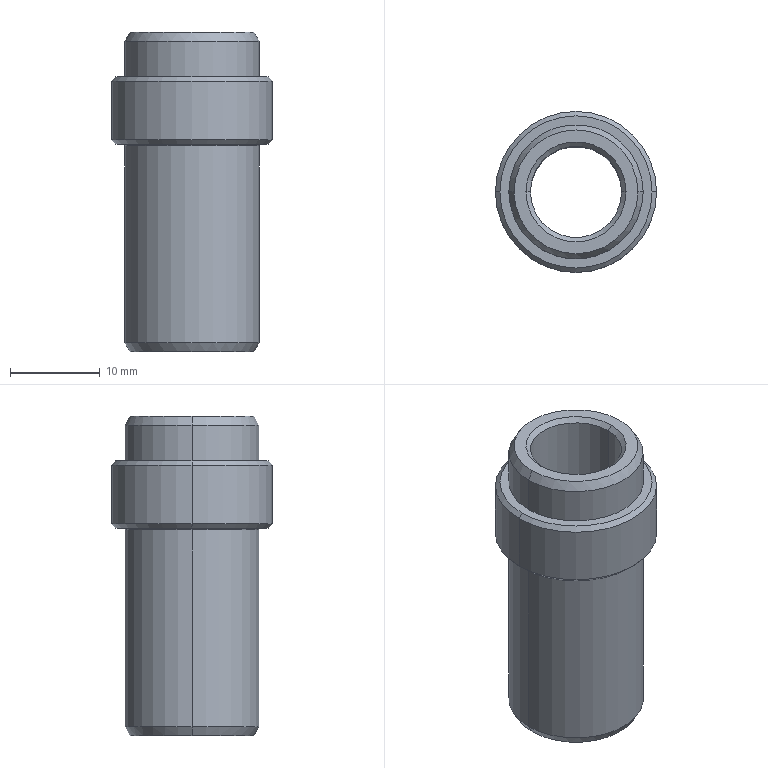Part | STEP file | PLACA BASE EXCENTRICA | 1 solid | 26 faces | box 18 x 18 x 35.7 mm | volume 3926 mm3 | cone 12 | cylinder 8 | plane 4 | torus 2 | commonest cylinder face diameters 15 x4 10.2 x2 18 x2
STEP:
#1=CARTESIAN_POINT('',(8.5,0.,-2.));
#2=VERTEX_POINT('',#1);
#3=CARTESIAN_POINT('',(-8.5,0.,-2.));
#4=VERTEX_POINT('',#3);
#5=CARTESIAN_POINT('',(0.,0.,-2.));
#6=DIRECTION('',(0.,0.,1.));
#7=DIRECTION('',(1.,0.,0.));
#8=AXIS2_PLACEMENT_3D('',#5,#6,#7);
#9=CIRCLE('',#8,8.5);
#10=EDGE_CURVE('',#2,#4,#9,.T.);
#11=ORIENTED_EDGE('',*,*,#10,.F.);
#12=CARTESIAN_POINT('',(9.,0.,-2.5));
#13=VERTEX_POINT('',#12);
#14=CARTESIAN_POINT('',(9.,0.,-2.5));
#15=DIRECTION('',(0.7071,0.,-0.7071));
#16=VECTOR('',#15,1000.);
#17=LINE('',#14,#16);
#18=EDGE_CURVE('',#2,#13,#17,.T.);
#19=ORIENTED_EDGE('',*,*,#18,.T.);
#20=CARTESIAN_POINT('',(-9.,0.,-2.5));
#21=VERTEX_POINT('',#20);
#22=CARTESIAN_POINT('',(0.,0.,-2.5));
#23=DIRECTION('',(0.,0.,-1.));
#24=DIRECTION('',(1.,0.,0.));
#25=AXIS2_PLACEMENT_3D('',#22,#23,#24);
#26=CIRCLE('',#25,9.);
#27=EDGE_CURVE('',#21,#13,#26,.T.);
#28=ORIENTED_EDGE('',*,*,#27,.F.);
#29=CARTESIAN_POINT('',(-9.,0.,-2.5));
#30=DIRECTION('',(-0.7071,0.,-0.7071));
#31=VECTOR('',#30,1000.);
#32=LINE('',#29,#31);
#33=EDGE_CURVE('',#4,#21,#32,.T.);
#34=ORIENTED_EDGE('',*,*,#33,.F.);
#35=EDGE_LOOP('',(#11,#19,#28,#34));
#36=FACE_OUTER_BOUND('',#35,.T.);
#37=CARTESIAN_POINT('',(0.,0.,-2.5));
#38=DIRECTION('',(0.,0.,-1.));
#39=DIRECTION('',(-1.,0.,0.));
#40=AXIS2_PLACEMENT_3D('',#37,#38,#39);
#41=CONICAL_SURFACE('',#40,9.,0.7854);
#42=ADVANCED_FACE('',(#36),#41,.T.);
#43=CARTESIAN_POINT('',(-8.5,0.,-9.5));
#44=VERTEX_POINT('',#43);
#45=CARTESIAN_POINT('',(8.5,0.,-9.5));
#46=VERTEX_POINT('',#45);
#47=CARTESIAN_POINT('',(0.,0.,-9.5));
#48=DIRECTION('',(0.,0.,-1.));
#49=DIRECTION('',(-1.,0.,0.));
#50=AXIS2_PLACEMENT_3D('',#47,#48,#49);
#51=CIRCLE('',#50,8.5);
#52=EDGE_CURVE('',#44,#46,#51,.T.);
#53=ORIENTED_EDGE('',*,*,#52,.F.);
#54=CARTESIAN_POINT('',(-9.,0.,-9.));
#55=VERTEX_POINT('',#54);
#56=CARTESIAN_POINT('',(-8.5,0.,-9.5));
#57=DIRECTION('',(-0.7071,0.,0.7071));
#58=VECTOR('',#57,1000.);
#59=LINE('',#56,#58);
#60=EDGE_CURVE('',#44,#55,#59,.T.);
#61=ORIENTED_EDGE('',*,*,#60,.T.);
#62=CARTESIAN_POINT('',(9.,0.,-9.));
#63=VERTEX_POINT('',#62);
#64=CARTESIAN_POINT('',(0.,0.,-9.));
#65=DIRECTION('',(0.,0.,1.));
#66=DIRECTION('',(-1.,0.,0.));
#67=AXIS2_PLACEMENT_3D('',#64,#65,#66);
#68=CIRCLE('',#67,9.);
#69=EDGE_CURVE('',#63,#55,#68,.T.);
#70=ORIENTED_EDGE('',*,*,#69,.F.);
#71=CARTESIAN_POINT('',(8.5,0.,-9.5));
#72=DIRECTION('',(0.7071,0.,0.7071));
#73=VECTOR('',#72,1000.);
#74=LINE('',#71,#73);
#75=EDGE_CURVE('',#46,#63,#74,.T.);
#76=ORIENTED_EDGE('',*,*,#75,.F.);
#77=EDGE_LOOP('',(#53,#61,#70,#76));
#78=FACE_OUTER_BOUND('',#77,.T.);
#79=CARTESIAN_POINT('',(0.,0.,-9.5));
#80=DIRECTION('',(0.,0.,1.));
#81=DIRECTION('',(1.,0.,0.));
#82=AXIS2_PLACEMENT_3D('',#79,#80,#81);
#83=CONICAL_SURFACE('',#82,8.5,0.7854);
#84=ADVANCED_FACE('',(#78),#83,.T.);
#85=CARTESIAN_POINT('',(6.923,0.,3.));
#86=VERTEX_POINT('',#85);
#87=CARTESIAN_POINT('',(-6.923,0.,3.));
#88=VERTEX_POINT('',#87);
#89=CARTESIAN_POINT('',(0.,0.,3.));
#90=DIRECTION('',(0.,0.,1.));
#91=DIRECTION('',(1.,0.,0.));
#92=AXIS2_PLACEMENT_3D('',#89,#90,#91);
#93=CIRCLE('',#92,6.923);
#94=EDGE_CURVE('',#86,#88,#93,.T.);
#95=ORIENTED_EDGE('',*,*,#94,.F.);
#96=CARTESIAN_POINT('',(7.5,0.,2.));
#97=VERTEX_POINT('',#96);
#98=CARTESIAN_POINT('',(6.923,0.,3.));
#99=DIRECTION('',(0.5,0.,-0.866));
#100=VECTOR('',#99,1000.);
#101=LINE('',#98,#100);
#102=EDGE_CURVE('',#86,#97,#101,.T.);
#103=ORIENTED_EDGE('',*,*,#102,.T.);
#104=CARTESIAN_POINT('',(-7.5,0.,2.));
#105=VERTEX_POINT('',#104);
#106=CARTESIAN_POINT('',(0.,0.,2.));
#107=DIRECTION('',(0.,0.,-1.));
#108=DIRECTION('',(1.,0.,0.));
#109=AXIS2_PLACEMENT_3D('',#106,#107,#108);
#110=CIRCLE('',#109,7.5);
#111=EDGE_CURVE('',#105,#97,#110,.T.);
#112=ORIENTED_EDGE('',*,*,#111,.F.);
#113=CARTESIAN_POINT('',(-6.923,0.,3.));
#114=DIRECTION('',(-0.5,0.,-0.866));
#115=VECTOR('',#114,1000.);
#116=LINE('',#113,#115);
#117=EDGE_CURVE('',#88,#105,#116,.T.);
#118=ORIENTED_EDGE('',*,*,#117,.F.);
#119=EDGE_LOOP('',(#95,#103,#112,#118));
#120=FACE_OUTER_BOUND('',#119,.T.);
#121=CARTESIAN_POINT('',(0.,0.,3.));
#122=DIRECTION('',(0.,0.,-1.));
#123=DIRECTION('',(-1.,0.,0.));
#124=AXIS2_PLACEMENT_3D('',#121,#122,#123);
#125=CONICAL_SURFACE('',#124,6.923,0.5236);
#126=ADVANCED_FACE('',(#120),#125,.T.);
#127=CARTESIAN_POINT('',(-5.1,0.,2.5));
#128=VERTEX_POINT('',#127);
#129=CARTESIAN_POINT('',(5.1,0.,2.5));
#130=VERTEX_POINT('',#129);
#131=CARTESIAN_POINT('',(0.,0.,2.5));
#132=DIRECTION('',(0.,0.,1.));
#133=DIRECTION('',(1.,0.,0.));
#134=AXIS2_PLACEMENT_3D('',#131,#132,#133);
#135=CIRCLE('',#134,5.1);
#136=EDGE_CURVE('',#128,#130,#135,.T.);
#137=ORIENTED_EDGE('',*,*,#136,.F.);
#138=CARTESIAN_POINT('',(-5.6,0.,3.));
#139=VERTEX_POINT('',#138);
#140=CARTESIAN_POINT('',(-5.6,0.,3.));
#141=DIRECTION('',(-0.7071,0.,0.7071));
#142=VECTOR('',#141,1000.);
#143=LINE('',#140,#142);
#144=EDGE_CURVE('',#128,#139,#143,.T.);
#145=ORIENTED_EDGE('',*,*,#144,.T.);
#146=CARTESIAN_POINT('',(5.6,0.,3.));
#147=VERTEX_POINT('',#146);
#148=CARTESIAN_POINT('',(0.,0.,3.));
#149=DIRECTION('',(0.,0.,-1.));
#150=DIRECTION('',(1.,0.,0.));
#151=AXIS2_PLACEMENT_3D('',#148,#149,#150);
#152=CIRCLE('',#151,5.6);
#153=EDGE_CURVE('',#147,#139,#152,.T.);
#154=ORIENTED_EDGE('',*,*,#153,.F.);
#155=CARTESIAN_POINT('',(5.6,0.,3.));
#156=DIRECTION('',(0.7071,0.,0.7071));
#157=VECTOR('',#156,1000.);
#158=LINE('',#155,#157);
#159=EDGE_CURVE('',#130,#147,#158,.T.);
#160=ORIENTED_EDGE('',*,*,#159,.F.);
#161=EDGE_LOOP('',(#137,#145,#154,#160));
#162=FACE_OUTER_BOUND('',#161,.T.);
#163=CARTESIAN_POINT('',(0.,0.,3.));
#164=DIRECTION('',(0.,0.,1.));
#165=DIRECTION('',(1.,0.,0.));
#166=AXIS2_PLACEMENT_3D('',#163,#164,#165);
#167=CONICAL_SURFACE('',#166,5.6,0.7854);
#168=ADVANCED_FACE('',(#162),#167,.F.);
#169=CARTESIAN_POINT('',(5.1,0.,-32.2));
#170=VERTEX_POINT('',#169);
#171=CARTESIAN_POINT('',(-5.1,0.,-32.2));
#172=VERTEX_POINT('',#171);
#173=CARTESIAN_POINT('',(0.,0.,-32.2));
#174=DIRECTION('',(0.,0.,-1.));
#175=DIRECTION('',(1.,0.,0.));
#176=AXIS2_PLACEMENT_3D('',#173,#174,#175);
#177=CIRCLE('',#176,5.1);
#178=EDGE_CURVE('',#170,#172,#177,.T.);
#179=ORIENTED_EDGE('',*,*,#178,.F.);
#180=CARTESIAN_POINT('',(5.6,0.,-32.7));
#181=VERTEX_POINT('',#180);
#182=CARTESIAN_POINT('',(5.1,0.,-32.2));
#183=DIRECTION('',(0.7071,0.,-0.7071));
#184=VECTOR('',#183,1000.);
#185=LINE('',#182,#184);
#186=EDGE_CURVE('',#170,#181,#185,.T.);
#187=ORIENTED_EDGE('',*,*,#186,.T.);
#188=CARTESIAN_POINT('',(-5.6,0.,-32.7));
#189=VERTEX_POINT('',#188);
#190=CARTESIAN_POINT('',(0.,0.,-32.7));
#191=DIRECTION('',(0.,0.,1.));
#192=DIRECTION('',(1.,0.,0.));
#193=AXIS2_PLACEMENT_3D('',#190,#191,#192);
#194=CIRCLE('',#193,5.6);
#195=EDGE_CURVE('',#189,#181,#194,.T.);
#196=ORIENTED_EDGE('',*,*,#195,.F.);
#197=CARTESIAN_POINT('',(-5.1,0.,-32.2));
#198=DIRECTION('',(-0.7071,0.,-0.7071));
#199=VECTOR('',#198,1000.);
#200=LINE('',#197,#199);
#201=EDGE_CURVE('',#172,#189,#200,.T.);
#202=ORIENTED_EDGE('',*,*,#201,.F.);
#203=EDGE_LOOP('',(#179,#187,#196,#202));
#204=FACE_OUTER_BOUND('',#203,.T.);
#205=CARTESIAN_POINT('',(0.,0.,-32.2));
#206=DIRECTION('',(0.,0.,-1.));
#207=DIRECTION('',(-1.,0.,0.));
#208=AXIS2_PLACEMENT_3D('',#205,#206,#207);
#209=CONICAL_SURFACE('',#208,5.1,0.7854);
#210=ADVANCED_FACE('',(#204),#209,.F.);
#211=ORIENTED_EDGE('',*,*,#136,.T.);
#212=CARTESIAN_POINT('',(5.1,0.,-32.7));
#213=DIRECTION('',(0.,0.,-1.));
#214=VECTOR('',#213,1000.);
#215=LINE('',#212,#214);
#216=EDGE_CURVE('',#130,#170,#215,.T.);
#217=ORIENTED_EDGE('',*,*,#216,.T.);
#218=ORIENTED_EDGE('',*,*,#178,.T.);
#219=CARTESIAN_POINT('',(-5.1,0.,-32.7));
#220=DIRECTION('',(0.,0.,-1.));
#221=VECTOR('',#220,1000.);
#222=LINE('',#219,#221);
#223=EDGE_CURVE('',#128,#172,#222,.T.);
#224=ORIENTED_EDGE('',*,*,#223,.F.);
#225=EDGE_LOOP('',(#211,#217,#218,#224));
#226=FACE_OUTER_BOUND('',#225,.T.);
#227=CARTESIAN_POINT('',(0.,0.,-32.7));
#228=DIRECTION('',(0.,0.,-1.));
#229=DIRECTION('',(-1.,0.,0.));
#230=AXIS2_PLACEMENT_3D('',#227,#228,#229);
#231=CYLINDRICAL_SURFACE('',#230,5.1);
#232=ADVANCED_FACE('',(#226),#231,.F.);
#233=CARTESIAN_POINT('',(-6.923,0.,-32.7));
#234=VERTEX_POINT('',#233);
#235=CARTESIAN_POINT('',(6.923,0.,-32.7));
#236=VERTEX_POINT('',#235);
#237=CARTESIAN_POINT('',(0.,0.,-32.7));
#238=DIRECTION('',(0.,0.,-1.));
#239=DIRECTION('',(1.,0.,0.));
#240=AXIS2_PLACEMENT_3D('',#237,#238,#239);
#241=CIRCLE('',#240,6.923);
#242=EDGE_CURVE('',#234,#236,#241,.T.);
#243=ORIENTED_EDGE('',*,*,#242,.F.);
#244=CARTESIAN_POINT('',(-7.5,0.,-31.7));
#245=VERTEX_POINT('',#244);
#246=CARTESIAN_POINT('',(-7.5,0.,-31.7));
#247=DIRECTION('',(-0.5,0.,0.866));
#248=VECTOR('',#247,1000.);
#249=LINE('',#246,#248);
#250=EDGE_CURVE('',#234,#245,#249,.T.);
#251=ORIENTED_EDGE('',*,*,#250,.T.);
#252=CARTESIAN_POINT('',(7.5,0.,-31.7));
#253=VERTEX_POINT('',#252);
#254=CARTESIAN_POINT('',(0.,0.,-31.7));
#255=DIRECTION('',(0.,0.,1.));
#256=DIRECTION('',(1.,0.,0.));
#257=AXIS2_PLACEMENT_3D('',#254,#255,#256);
#258=CIRCLE('',#257,7.5);
#259=EDGE_CURVE('',#253,#245,#258,.T.);
#260=ORIENTED_EDGE('',*,*,#259,.F.);
#261=CARTESIAN_POINT('',(7.5,0.,-31.7));
#262=DIRECTION('',(0.5,0.,0.866));
#263=VECTOR('',#262,1000.);
#264=LINE('',#261,#263);
#265=EDGE_CURVE('',#236,#253,#264,.T.);
#266=ORIENTED_EDGE('',*,*,#265,.F.);
#267=EDGE_LOOP('',(#243,#251,#260,#266));
#268=FACE_OUTER_BOUND('',#267,.T.);
#269=CARTESIAN_POINT('',(0.,0.,-31.7));
#270=DIRECTION('',(0.,0.,1.));
#271=DIRECTION('',(1.,0.,0.));
#272=AXIS2_PLACEMENT_3D('',#269,#270,#271);
#273=CONICAL_SURFACE('',#272,7.5,0.5236);
#274=ADVANCED_FACE('',(#268),#273,.T.);
#275=CARTESIAN_POINT('',(7.5,0.,-9.7));
#276=VERTEX_POINT('',#275);
#277=CARTESIAN_POINT('',(-7.5,0.,-9.7));
#278=VERTEX_POINT('',#277);
#279=CARTESIAN_POINT('',(0.,0.,-9.7));
#280=DIRECTION('',(0.,0.,-1.));
#281=DIRECTION('',(-1.,0.,0.));
#282=AXIS2_PLACEMENT_3D('',#279,#280,#281);
#283=CIRCLE('',#282,7.5);
#284=EDGE_CURVE('',#276,#278,#283,.T.);
#285=ORIENTED_EDGE('',*,*,#284,.F.);
#286=CARTESIAN_POINT('',(7.7,0.,-9.5));
#287=VERTEX_POINT('',#286);
#288=CARTESIAN_POINT('',(7.7,0.,-9.7));
#289=DIRECTION('',(0.,1.,0.));
#290=DIRECTION('',(-1.,0.,0.));
#291=AXIS2_PLACEMENT_3D('',#288,#289,#290);
#292=CIRCLE('',#291,0.2);
#293=EDGE_CURVE('',#276,#287,#292,.T.);
#294=ORIENTED_EDGE('',*,*,#293,.T.);
#295=CARTESIAN_POINT('',(-7.7,0.,-9.5));
#296=VERTEX_POINT('',#295);
#297=CARTESIAN_POINT('',(0.,0.,-9.5));
#298=DIRECTION('',(0.,0.,1.));
#299=DIRECTION('',(-1.,0.,0.));
#300=AXIS2_PLACEMENT_3D('',#297,#298,#299);
#301=CIRCLE('',#300,7.7);
#302=EDGE_CURVE('',#296,#287,#301,.T.);
#303=ORIENTED_EDGE('',*,*,#302,.F.);
#304=CARTESIAN_POINT('',(-7.7,0.,-9.7));
#305=DIRECTION('',(0.,-1.,0.));
#306=DIRECTION('',(0.,0.,-1.));
#307=AXIS2_PLACEMENT_3D('',#304,#305,#306);
#308=CIRCLE('',#307,0.2);
#309=EDGE_CURVE('',#278,#296,#308,.T.);
#310=ORIENTED_EDGE('',*,*,#309,.F.);
#311=EDGE_LOOP('',(#285,#294,#303,#310));
#312=FACE_OUTER_BOUND('',#311,.T.);
#313=CARTESIAN_POINT('',(0.,0.,-9.7));
#314=DIRECTION('',(0.,0.,-1.));
#315=DIRECTION('',(-1.,0.,0.));
#316=AXIS2_PLACEMENT_3D('',#313,#314,#315);
#317=TOROIDAL_SURFACE('',#316,7.7,0.2);
#318=ADVANCED_FACE('',(#312),#317,.F.);
#319=ORIENTED_EDGE('',*,*,#259,.T.);
#320=CARTESIAN_POINT('',(-7.5,0.,-32.7));
#321=DIRECTION('',(0.,0.,1.));
#322=VECTOR('',#321,1000.);
#323=LINE('',#320,#322);
#324=EDGE_CURVE('',#245,#278,#323,.T.);
#325=ORIENTED_EDGE('',*,*,#324,.T.);
#326=CARTESIAN_POINT('',(0.,0.,-9.7));
#327=DIRECTION('',(0.,0.,-1.));
#328=DIRECTION('',(-1.,0.,0.));
#329=AXIS2_PLACEMENT_3D('',#326,#327,#328);
#330=CIRCLE('',#329,7.5);
#331=EDGE_CURVE('',#278,#276,#330,.T.);
#332=ORIENTED_EDGE('',*,*,#331,.T.);
#333=CARTESIAN_POINT('',(7.5,0.,-32.7));
#334=DIRECTION('',(0.,0.,1.));
#335=VECTOR('',#334,1000.);
#336=LINE('',#333,#335);
#337=EDGE_CURVE('',#253,#276,#336,.T.);
#338=ORIENTED_EDGE('',*,*,#337,.F.);
#339=EDGE_LOOP('',(#319,#325,#332,#338));
#340=FACE_OUTER_BOUND('',#339,.T.);
#341=CARTESIAN_POINT('',(0.,0.,-32.7));
#342=DIRECTION('',(0.,0.,1.));
#343=DIRECTION('',(1.,0.,0.));
#344=AXIS2_PLACEMENT_3D('',#341,#342,#343);
#345=CYLINDRICAL_SURFACE('',#344,7.5);
#346=ADVANCED_FACE('',(#340),#345,.T.);
#347=ORIENTED_EDGE('',*,*,#27,.T.);
#348=CARTESIAN_POINT('',(9.,0.,-9.5));
#349=DIRECTION('',(0.,0.,-1.));
#350=VECTOR('',#349,1000.);
#351=LINE('',#348,#350);
#352=EDGE_CURVE('',#13,#63,#351,.T.);
#353=ORIENTED_EDGE('',*,*,#352,.T.);
#354=ORIENTED_EDGE('',*,*,#69,.T.);
#355=CARTESIAN_POINT('',(-9.,0.,-9.5));
#356=DIRECTION('',(0.,0.,-1.));
#357=VECTOR('',#356,1000.);
#358=LINE('',#355,#357);
#359=EDGE_CURVE('',#21,#55,#358,.T.);
#360=ORIENTED_EDGE('',*,*,#359,.F.);
#361=EDGE_LOOP('',(#347,#353,#354,#360));
#362=FACE_OUTER_BOUND('',#361,.T.);
#363=CARTESIAN_POINT('',(0.,0.,-9.5));
#364=DIRECTION('',(0.,0.,-1.));
#365=DIRECTION('',(-1.,0.,0.));
#366=AXIS2_PLACEMENT_3D('',#363,#364,#365);
#367=CYLINDRICAL_SURFACE('',#366,9.);
#368=ADVANCED_FACE('',(#362),#367,.T.);
#369=CARTESIAN_POINT('',(-7.5,0.,-2.));
#370=VERTEX_POINT('',#369);
#371=CARTESIAN_POINT('',(7.5,0.,-2.));
#372=VERTEX_POINT('',#371);
#373=CARTESIAN_POINT('',(0.,0.,-2.));
#374=DIRECTION('',(0.,0.,-1.));
#375=DIRECTION('',(1.,0.,0.));
#376=AXIS2_PLACEMENT_3D('',#373,#374,#375);
#377=CIRCLE('',#376,7.5);
#378=EDGE_CURVE('',#370,#372,#377,.T.);
#379=ORIENTED_EDGE('',*,*,#378,.F.);
#380=CARTESIAN_POINT('',(-7.5,0.,-32.7));
#381=DIRECTION('',(0.,0.,1.));
#382=VECTOR('',#381,1000.);
#383=LINE('',#380,#382);
#384=EDGE_CURVE('',#370,#105,#383,.T.);
#385=ORIENTED_EDGE('',*,*,#384,.T.);
#386=ORIENTED_EDGE('',*,*,#111,.T.);
#387=CARTESIAN_POINT('',(7.5,0.,-32.7));
#388=DIRECTION('',(0.,0.,1.));
#389=VECTOR('',#388,1000.);
#390=LINE('',#387,#389);
#391=EDGE_CURVE('',#372,#97,#390,.T.);
#392=ORIENTED_EDGE('',*,*,#391,.F.);
#393=EDGE_LOOP('',(#379,#385,#386,#392));
#394=FACE_OUTER_BOUND('',#393,.T.);
#395=CARTESIAN_POINT('',(0.,0.,-32.7));
#396=DIRECTION('',(0.,0.,1.));
#397=DIRECTION('',(1.,0.,0.));
#398=AXIS2_PLACEMENT_3D('',#395,#396,#397);
#399=CYLINDRICAL_SURFACE('',#398,7.5);
#400=ADVANCED_FACE('',(#394),#399,.T.);
#401=ORIENTED_EDGE('',*,*,#195,.T.);
#402=CARTESIAN_POINT('',(0.,0.,-32.7));
#403=DIRECTION('',(0.,0.,1.));
#404=DIRECTION('',(1.,0.,0.));
#405=AXIS2_PLACEMENT_3D('',#402,#403,#404);
#406=CIRCLE('',#405,5.6);
#407=EDGE_CURVE('',#181,#189,#406,.T.);
#408=ORIENTED_EDGE('',*,*,#407,.T.);
#409=EDGE_LOOP('',(#401,#408));
#410=FACE_BOUND('',#409,.T.);
#411=CARTESIAN_POINT('',(0.,0.,-32.7));
#412=DIRECTION('',(0.,0.,-1.));
#413=DIRECTION('',(1.,0.,0.));
#414=AXIS2_PLACEMENT_3D('',#411,#412,#413);
#415=CIRCLE('',#414,6.923);
#416=EDGE_CURVE('',#236,#234,#415,.T.);
#417=ORIENTED_EDGE('',*,*,#416,.T.);
#418=ORIENTED_EDGE('',*,*,#242,.T.);
#419=EDGE_LOOP('',(#417,#418));
#420=FACE_OUTER_BOUND('',#419,.T.);
#421=CARTESIAN_POINT('',(0.,0.,-32.7));
#422=DIRECTION('',(0.,0.,1.));
#423=DIRECTION('',(1.,0.,0.));
#424=AXIS2_PLACEMENT_3D('',#421,#422,#423);
#425=PLANE('',#424);
#426=ADVANCED_FACE('',(#410,#420),#425,.F.);
#427=ORIENTED_EDGE('',*,*,#384,.F.);
#428=CARTESIAN_POINT('',(0.,0.,-2.));
#429=DIRECTION('',(0.,0.,-1.));
#430=DIRECTION('',(1.,0.,0.));
#431=AXIS2_PLACEMENT_3D('',#428,#429,#430);
#432=CIRCLE('',#431,7.5);
#433=EDGE_CURVE('',#372,#370,#432,.T.);
#434=ORIENTED_EDGE('',*,*,#433,.F.);
#435=ORIENTED_EDGE('',*,*,#391,.T.);
#436=CARTESIAN_POINT('',(0.,0.,2.));
#437=DIRECTION('',(0.,0.,-1.));
#438=DIRECTION('',(1.,0.,0.));
#439=AXIS2_PLACEMENT_3D('',#436,#437,#438);
#440=CIRCLE('',#439,7.5);
#441=EDGE_CURVE('',#97,#105,#440,.T.);
#442=ORIENTED_EDGE('',*,*,#441,.T.);
#443=EDGE_LOOP('',(#427,#434,#435,#442));
#444=FACE_OUTER_BOUND('',#443,.T.);
#445=CARTESIAN_POINT('',(0.,0.,-32.7));
#446=DIRECTION('',(0.,0.,1.));
#447=DIRECTION('',(1.,0.,0.));
#448=AXIS2_PLACEMENT_3D('',#445,#446,#447);
#449=CYLINDRICAL_SURFACE('',#448,7.5);
#450=ADVANCED_FACE('',(#444),#449,.T.);
#451=CARTESIAN_POINT('',(0.,0.,3.));
#452=DIRECTION('',(0.,0.,1.));
#453=DIRECTION('',(1.,0.,0.));
#454=AXIS2_PLACEMENT_3D('',#451,#452,#453);
#455=CIRCLE('',#454,6.923);
#456=EDGE_CURVE('',#88,#86,#455,.T.);
#457=ORIENTED_EDGE('',*,*,#456,.T.);
#458=ORIENTED_EDGE('',*,*,#94,.T.);
#459=EDGE_LOOP('',(#457,#458));
#460=FACE_OUTER_BOUND('',#459,.T.);
#461=ORIENTED_EDGE('',*,*,#153,.T.);
#462=CARTESIAN_POINT('',(0.,0.,3.));
#463=DIRECTION('',(0.,0.,-1.));
#464=DIRECTION('',(1.,0.,0.));
#465=AXIS2_PLACEMENT_3D('',#462,#463,#464);
#466=CIRCLE('',#465,5.6);
#467=EDGE_CURVE('',#139,#147,#466,.T.);
#468=ORIENTED_EDGE('',*,*,#467,.T.);
#469=EDGE_LOOP('',(#461,#468));
#470=FACE_BOUND('',#469,.T.);
#471=CARTESIAN_POINT('',(0.,0.,3.));
#472=DIRECTION('',(0.,0.,1.));
#473=DIRECTION('',(1.,0.,0.));
#474=AXIS2_PLACEMENT_3D('',#471,#472,#473);
#475=PLANE('',#474);
#476=ADVANCED_FACE('',(#460,#470),#475,.T.);
#477=CARTESIAN_POINT('',(0.,0.,-2.));
#478=DIRECTION('',(0.,0.,1.));
#479=DIRECTION('',(1.,0.,0.));
#480=AXIS2_PLACEMENT_3D('',#477,#478,#479);
#481=CIRCLE('',#480,8.5);
#482=EDGE_CURVE('',#4,#2,#481,.T.);
#483=ORIENTED_EDGE('',*,*,#482,.T.);
#484=ORIENTED_EDGE('',*,*,#10,.T.);
#485=EDGE_LOOP('',(#483,#484));
#486=FACE_OUTER_BOUND('',#485,.T.);
#487=ORIENTED_EDGE('',*,*,#433,.T.);
#488=ORIENTED_EDGE('',*,*,#378,.T.);
#489=EDGE_LOOP('',(#487,#488));
#490=FACE_BOUND('',#489,.T.);
#491=CARTESIAN_POINT('',(0.,0.,-2.));
#492=DIRECTION('',(0.,0.,1.));
#493=DIRECTION('',(1.,0.,0.));
#494=AXIS2_PLACEMENT_3D('',#491,#492,#493);
#495=PLANE('',#494);
#496=ADVANCED_FACE('',(#486,#490),#495,.T.);
#497=ORIENTED_EDGE('',*,*,#352,.F.);
#498=CARTESIAN_POINT('',(0.,0.,-2.5));
#499=DIRECTION('',(0.,0.,-1.));
#500=DIRECTION('',(1.,0.,0.));
#501=AXIS2_PLACEMENT_3D('',#498,#499,#500);
#502=CIRCLE('',#501,9.);
#503=EDGE_CURVE('',#13,#21,#502,.T.);
#504=ORIENTED_EDGE('',*,*,#503,.T.);
#505=ORIENTED_EDGE('',*,*,#359,.T.);
#506=CARTESIAN_POINT('',(0.,0.,-9.));
#507=DIRECTION('',(0.,0.,1.));
#508=DIRECTION('',(-1.,0.,0.));
#509=AXIS2_PLACEMENT_3D('',#506,#507,#508);
#510=CIRCLE('',#509,9.);
#511=EDGE_CURVE('',#55,#63,#510,.T.);
#512=ORIENTED_EDGE('',*,*,#511,.T.);
#513=EDGE_LOOP('',(#497,#504,#505,#512));
#514=FACE_OUTER_BOUND('',#513,.T.);
#515=CARTESIAN_POINT('',(0.,0.,-9.5));
#516=DIRECTION('',(0.,0.,-1.));
#517=DIRECTION('',(-1.,0.,0.));
#518=AXIS2_PLACEMENT_3D('',#515,#516,#517);
#519=CYLINDRICAL_SURFACE('',#518,9.);
#520=ADVANCED_FACE('',(#514),#519,.T.);
#521=CARTESIAN_POINT('',(0.,0.,-9.5));
#522=DIRECTION('',(0.,0.,-1.));
#523=DIRECTION('',(-1.,0.,0.));
#524=AXIS2_PLACEMENT_3D('',#521,#522,#523);
#525=CIRCLE('',#524,8.5);
#526=EDGE_CURVE('',#46,#44,#525,.T.);
#527=ORIENTED_EDGE('',*,*,#526,.T.);
#528=ORIENTED_EDGE('',*,*,#52,.T.);
#529=EDGE_LOOP('',(#527,#528));
#530=FACE_OUTER_BOUND('',#529,.T.);
#531=ORIENTED_EDGE('',*,*,#302,.T.);
#532=CARTESIAN_POINT('',(0.,0.,-9.5));
#533=DIRECTION('',(0.,0.,1.));
#534=DIRECTION('',(-1.,0.,0.));
#535=AXIS2_PLACEMENT_3D('',#532,#533,#534);
#536=CIRCLE('',#535,7.7);
#537=EDGE_CURVE('',#287,#296,#536,.T.);
#538=ORIENTED_EDGE('',*,*,#537,.T.);
#539=EDGE_LOOP('',(#531,#538));
#540=FACE_BOUND('',#539,.T.);
#541=CARTESIAN_POINT('',(0.,9.,-9.5));
#542=DIRECTION('',(0.,0.,-1.));
#543=DIRECTION('',(-1.,0.,0.));
#544=AXIS2_PLACEMENT_3D('',#541,#542,#543);
#545=PLANE('',#544);
#546=ADVANCED_FACE('',(#530,#540),#545,.T.);
#547=ORIENTED_EDGE('',*,*,#324,.F.);
#548=CARTESIAN_POINT('',(0.,0.,-31.7));
#549=DIRECTION('',(0.,0.,1.));
#550=DIRECTION('',(1.,0.,0.));
#551=AXIS2_PLACEMENT_3D('',#548,#549,#550);
#552=CIRCLE('',#551,7.5);
#553=EDGE_CURVE('',#245,#253,#552,.T.);
#554=ORIENTED_EDGE('',*,*,#553,.T.);
#555=ORIENTED_EDGE('',*,*,#337,.T.);
#556=ORIENTED_EDGE('',*,*,#284,.T.);
#557=EDGE_LOOP('',(#547,#554,#555,#556));
#558=FACE_OUTER_BOUND('',#557,.T.);
#559=CARTESIAN_POINT('',(0.,0.,-32.7));
#560=DIRECTION('',(0.,0.,1.));
#561=DIRECTION('',(1.,0.,0.));
#562=AXIS2_PLACEMENT_3D('',#559,#560,#561);
#563=CYLINDRICAL_SURFACE('',#562,7.5);
#564=ADVANCED_FACE('',(#558),#563,.T.);
#565=ORIENTED_EDGE('',*,*,#293,.F.);
#566=ORIENTED_EDGE('',*,*,#331,.F.);
#567=ORIENTED_EDGE('',*,*,#309,.T.);
#568=ORIENTED_EDGE('',*,*,#537,.F.);
#569=EDGE_LOOP('',(#565,#566,#567,#568));
#570=FACE_OUTER_BOUND('',#569,.T.);
#571=CARTESIAN_POINT('',(0.,0.,-9.7));
#572=DIRECTION('',(0.,0.,-1.));
#573=DIRECTION('',(-1.,0.,0.));
#574=AXIS2_PLACEMENT_3D('',#571,#572,#573);
#575=TOROIDAL_SURFACE('',#574,7.7,0.2);
#576=ADVANCED_FACE('',(#570),#575,.F.);
#577=ORIENTED_EDGE('',*,*,#250,.F.);
#578=ORIENTED_EDGE('',*,*,#416,.F.);
#579=ORIENTED_EDGE('',*,*,#265,.T.);
#580=ORIENTED_EDGE('',*,*,#553,.F.);
#581=EDGE_LOOP('',(#577,#578,#579,#580));
#582=FACE_OUTER_BOUND('',#581,.T.);
#583=CARTESIAN_POINT('',(0.,0.,-31.7));
#584=DIRECTION('',(0.,0.,1.));
#585=DIRECTION('',(1.,0.,0.));
#586=AXIS2_PLACEMENT_3D('',#583,#584,#585);
#587=CONICAL_SURFACE('',#586,7.5,0.5236);
#588=ADVANCED_FACE('',(#582),#587,.T.);
#589=ORIENTED_EDGE('',*,*,#216,.F.);
#590=CARTESIAN_POINT('',(0.,0.,2.5));
#591=DIRECTION('',(0.,0.,1.));
#592=DIRECTION('',(1.,0.,0.));
#593=AXIS2_PLACEMENT_3D('',#590,#591,#592);
#594=CIRCLE('',#593,5.1);
#595=EDGE_CURVE('',#130,#128,#594,.T.);
#596=ORIENTED_EDGE('',*,*,#595,.T.);
#597=ORIENTED_EDGE('',*,*,#223,.T.);
#598=CARTESIAN_POINT('',(0.,0.,-32.2));
#599=DIRECTION('',(0.,0.,-1.));
#600=DIRECTION('',(1.,0.,0.));
#601=AXIS2_PLACEMENT_3D('',#598,#599,#600);
#602=CIRCLE('',#601,5.1);
#603=EDGE_CURVE('',#172,#170,#602,.T.);
#604=ORIENTED_EDGE('',*,*,#603,.T.);
#605=EDGE_LOOP('',(#589,#596,#597,#604));
#606=FACE_OUTER_BOUND('',#605,.T.);
#607=CARTESIAN_POINT('',(0.,0.,-32.7));
#608=DIRECTION('',(0.,0.,-1.));
#609=DIRECTION('',(-1.,0.,0.));
#610=AXIS2_PLACEMENT_3D('',#607,#608,#609);
#611=CYLINDRICAL_SURFACE('',#610,5.1);
#612=ADVANCED_FACE('',(#606),#611,.F.);
#613=ORIENTED_EDGE('',*,*,#186,.F.);
#614=ORIENTED_EDGE('',*,*,#603,.F.);
#615=ORIENTED_EDGE('',*,*,#201,.T.);
#616=ORIENTED_EDGE('',*,*,#407,.F.);
#617=EDGE_LOOP('',(#613,#614,#615,#616));
#618=FACE_OUTER_BOUND('',#617,.T.);
#619=CARTESIAN_POINT('',(0.,0.,-32.2));
#620=DIRECTION('',(0.,0.,-1.));
#621=DIRECTION('',(-1.,0.,0.));
#622=AXIS2_PLACEMENT_3D('',#619,#620,#621);
#623=CONICAL_SURFACE('',#622,5.1,0.7854);
#624=ADVANCED_FACE('',(#618),#623,.F.);
#625=ORIENTED_EDGE('',*,*,#144,.F.);
#626=ORIENTED_EDGE('',*,*,#595,.F.);
#627=ORIENTED_EDGE('',*,*,#159,.T.);
#628=ORIENTED_EDGE('',*,*,#467,.F.);
#629=EDGE_LOOP('',(#625,#626,#627,#628));
#630=FACE_OUTER_BOUND('',#629,.T.);
#631=CARTESIAN_POINT('',(0.,0.,3.));
#632=DIRECTION('',(0.,0.,1.));
#633=DIRECTION('',(1.,0.,0.));
#634=AXIS2_PLACEMENT_3D('',#631,#632,#633);
#635=CONICAL_SURFACE('',#634,5.6,0.7854);
#636=ADVANCED_FACE('',(#630),#635,.F.);
#637=ORIENTED_EDGE('',*,*,#102,.F.);
#638=ORIENTED_EDGE('',*,*,#456,.F.);
#639=ORIENTED_EDGE('',*,*,#117,.T.);
#640=ORIENTED_EDGE('',*,*,#441,.F.);
#641=EDGE_LOOP('',(#637,#638,#639,#640));
#642=FACE_OUTER_BOUND('',#641,.T.);
#643=CARTESIAN_POINT('',(0.,0.,3.));
#644=DIRECTION('',(0.,0.,-1.));
#645=DIRECTION('',(-1.,0.,0.));
#646=AXIS2_PLACEMENT_3D('',#643,#644,#645);
#647=CONICAL_SURFACE('',#646,6.923,0.5236);
#648=ADVANCED_FACE('',(#642),#647,.T.);
#649=ORIENTED_EDGE('',*,*,#60,.F.);
#650=ORIENTED_EDGE('',*,*,#526,.F.);
#651=ORIENTED_EDGE('',*,*,#75,.T.);
#652=ORIENTED_EDGE('',*,*,#511,.F.);
#653=EDGE_LOOP('',(#649,#650,#651,#652));
#654=FACE_OUTER_BOUND('',#653,.T.);
#655=CARTESIAN_POINT('',(0.,0.,-9.5));
#656=DIRECTION('',(0.,0.,1.));
#657=DIRECTION('',(1.,0.,0.));
#658=AXIS2_PLACEMENT_3D('',#655,#656,#657);
#659=CONICAL_SURFACE('',#658,8.5,0.7854);
#660=ADVANCED_FACE('',(#654),#659,.T.);
#661=ORIENTED_EDGE('',*,*,#18,.F.);
#662=ORIENTED_EDGE('',*,*,#482,.F.);
#663=ORIENTED_EDGE('',*,*,#33,.T.);
#664=ORIENTED_EDGE('',*,*,#503,.F.);
#665=EDGE_LOOP('',(#661,#662,#663,#664));
#666=FACE_OUTER_BOUND('',#665,.T.);
#667=CARTESIAN_POINT('',(0.,0.,-2.5));
#668=DIRECTION('',(0.,0.,-1.));
#669=DIRECTION('',(-1.,0.,0.));
#670=AXIS2_PLACEMENT_3D('',#667,#668,#669);
#671=CONICAL_SURFACE('',#670,9.,0.7854);
#672=ADVANCED_FACE('',(#666),#671,.T.);
#673=CLOSED_SHELL('',(#42,#84,#126,#168,#210,#232,#274,#318,#346,#368,#400,#426,#450,#476,#496,#520,#546,#564,#576,#588,#612,#624,#636,#648,#660,#672));
#674=MANIFOLD_SOLID_BREP('',#673);
#675=CARTESIAN_POINT('',(0.,0.,0.));
#676=DIRECTION('',(0.,0.,1.));
#677=DIRECTION('',(1.,0.,0.));
#678=AXIS2_PLACEMENT_3D('',#675,#676,#677);
#679=(LENGTH_UNIT()NAMED_UNIT(*)SI_UNIT(.MILLI.,.METRE.));
#680=UNCERTAINTY_MEASURE_WITH_UNIT(LENGTH_MEASURE(0.00001),#679,'','');
#681=(NAMED_UNIT(*)PLANE_ANGLE_UNIT()SI_UNIT($,.RADIAN.));
#682=(NAMED_UNIT(*)SI_UNIT($,.STERADIAN.)SOLID_ANGLE_UNIT());
#683=(GEOMETRIC_REPRESENTATION_CONTEXT(3)GLOBAL_UNCERTAINTY_ASSIGNED_CONTEXT((#680))GLOBAL_UNIT_ASSIGNED_CONTEXT((#679,#681,#682))REPRESENTATION_CONTEXT('',''));
#684=ADVANCED_BREP_SHAPE_REPRESENTATION('',(#674,#678),#683);